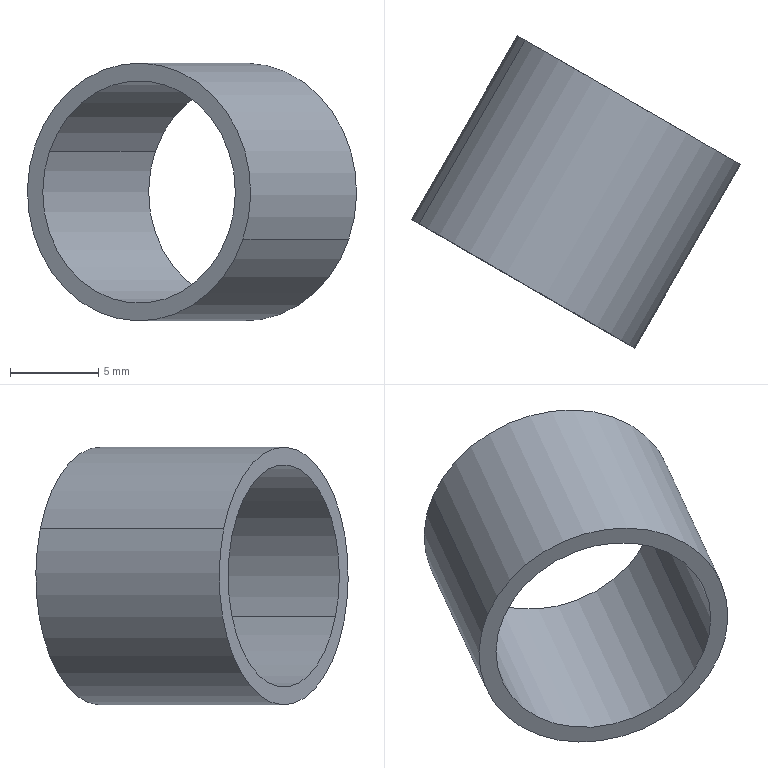Part | SolidWorks | features BaseBody 1 | 1 solid | 6 faces | box 18.644 x 17.692 x 14.6 mm | volume 512.708 mm3 | cylinder 4 | plane 2 | commonest cylinder face diameters 12.6 x2 14.6 x2
STEP:
#1=CARTESIAN_POINT('',(325.471,269.362,2.3));
#2=VERTEX_POINT('',#1);
#3=CARTESIAN_POINT('',(335.629,263.497,-2.3));
#4=VERTEX_POINT('',#3);
#5=CARTESIAN_POINT('',(330.55,266.429,0.));
#6=DIRECTION('',(-0.5,-0.866,0.));
#7=DIRECTION('',(0.8063,-0.4655,-0.365));
#8=AXIS2_PLACEMENT_3D('',#5,#6,#7);
#9=CIRCLE('',#8,6.3);
#10=EDGE_CURVE('',#2,#4,#9,.T.);
#11=ORIENTED_EDGE('',*,*,#10,.T.);
#12=CARTESIAN_POINT('',(341.629,273.889,-2.3));
#13=VERTEX_POINT('',#12);
#14=CARTESIAN_POINT('',(335.629,263.497,-2.3));
#15=DIRECTION('',(0.5,0.866,0.));
#16=VECTOR('',#15,1000.);
#17=LINE('',#14,#16);
#18=EDGE_CURVE('',#4,#13,#17,.T.);
#19=ORIENTED_EDGE('',*,*,#18,.T.);
#20=CARTESIAN_POINT('',(331.471,279.754,2.3));
#21=VERTEX_POINT('',#20);
#22=CARTESIAN_POINT('',(336.55,276.821,0.));
#23=DIRECTION('',(-0.5,-0.866,0.));
#24=DIRECTION('',(0.8063,-0.4655,-0.365));
#25=AXIS2_PLACEMENT_3D('',#22,#23,#24);
#26=CIRCLE('',#25,6.3);
#27=EDGE_CURVE('',#21,#13,#26,.T.);
#28=ORIENTED_EDGE('',*,*,#27,.F.);
#29=CARTESIAN_POINT('',(325.471,269.362,2.3));
#30=DIRECTION('',(0.5,0.866,0.));
#31=VECTOR('',#30,1000.);
#32=LINE('',#29,#31);
#33=EDGE_CURVE('',#2,#21,#32,.T.);
#34=ORIENTED_EDGE('',*,*,#33,.F.);
#35=EDGE_LOOP('',(#11,#19,#28,#34));
#36=FACE_OUTER_BOUND('',#35,.T.);
#37=CARTESIAN_POINT('',(330.55,266.429,0.));
#38=DIRECTION('',(0.5,0.866,0.));
#39=DIRECTION('',(-0.8063,0.4655,0.365));
#40=AXIS2_PLACEMENT_3D('',#37,#38,#39);
#41=CYLINDRICAL_SURFACE('',#40,6.3);
#42=ADVANCED_FACE('',(#36),#41,.F.);
#43=CARTESIAN_POINT('',(336.436,263.031,-2.665));
#44=VERTEX_POINT('',#43);
#45=CARTESIAN_POINT('',(324.664,269.827,2.665));
#46=VERTEX_POINT('',#45);
#47=CARTESIAN_POINT('',(330.55,266.429,0.));
#48=DIRECTION('',(-0.5,-0.866,0.));
#49=DIRECTION('',(0.8063,-0.4655,-0.365));
#50=AXIS2_PLACEMENT_3D('',#47,#48,#49);
#51=CIRCLE('',#50,7.3);
#52=EDGE_CURVE('',#44,#46,#51,.T.);
#53=ORIENTED_EDGE('',*,*,#52,.F.);
#54=CARTESIAN_POINT('',(342.436,273.423,-2.665));
#55=VERTEX_POINT('',#54);
#56=CARTESIAN_POINT('',(336.436,263.031,-2.665));
#57=DIRECTION('',(0.5,0.866,0.));
#58=VECTOR('',#57,1000.);
#59=LINE('',#56,#58);
#60=EDGE_CURVE('',#44,#55,#59,.T.);
#61=ORIENTED_EDGE('',*,*,#60,.T.);
#62=CARTESIAN_POINT('',(330.664,280.22,2.665));
#63=VERTEX_POINT('',#62);
#64=CARTESIAN_POINT('',(336.55,276.821,0.));
#65=DIRECTION('',(-0.5,-0.866,0.));
#66=DIRECTION('',(0.8063,-0.4655,-0.365));
#67=AXIS2_PLACEMENT_3D('',#64,#65,#66);
#68=CIRCLE('',#67,7.3);
#69=EDGE_CURVE('',#55,#63,#68,.T.);
#70=ORIENTED_EDGE('',*,*,#69,.T.);
#71=CARTESIAN_POINT('',(324.664,269.827,2.665));
#72=DIRECTION('',(0.5,0.866,0.));
#73=VECTOR('',#72,1000.);
#74=LINE('',#71,#73);
#75=EDGE_CURVE('',#46,#63,#74,.T.);
#76=ORIENTED_EDGE('',*,*,#75,.F.);
#77=EDGE_LOOP('',(#53,#61,#70,#76));
#78=FACE_OUTER_BOUND('',#77,.T.);
#79=CARTESIAN_POINT('',(330.55,266.429,0.));
#80=DIRECTION('',(0.5,0.866,0.));
#81=DIRECTION('',(-0.8063,0.4655,0.365));
#82=AXIS2_PLACEMENT_3D('',#79,#80,#81);
#83=CYLINDRICAL_SURFACE('',#82,7.3);
#84=ADVANCED_FACE('',(#78),#83,.T.);
#85=CARTESIAN_POINT('',(330.55,266.429,0.));
#86=DIRECTION('',(-0.5,-0.866,0.));
#87=DIRECTION('',(0.8063,-0.4655,-0.365));
#88=AXIS2_PLACEMENT_3D('',#85,#86,#87);
#89=CIRCLE('',#88,7.3);
#90=EDGE_CURVE('',#46,#44,#89,.T.);
#91=ORIENTED_EDGE('',*,*,#90,.T.);
#92=ORIENTED_EDGE('',*,*,#52,.T.);
#93=EDGE_LOOP('',(#91,#92));
#94=FACE_OUTER_BOUND('',#93,.T.);
#95=ORIENTED_EDGE('',*,*,#10,.F.);
#96=CARTESIAN_POINT('',(330.55,266.429,0.));
#97=DIRECTION('',(-0.5,-0.866,0.));
#98=DIRECTION('',(0.8063,-0.4655,-0.365));
#99=AXIS2_PLACEMENT_3D('',#96,#97,#98);
#100=CIRCLE('',#99,6.3);
#101=EDGE_CURVE('',#4,#2,#100,.T.);
#102=ORIENTED_EDGE('',*,*,#101,.F.);
#103=EDGE_LOOP('',(#95,#102));
#104=FACE_BOUND('',#103,.T.);
#105=CARTESIAN_POINT('',(330.55,266.429,0.));
#106=DIRECTION('',(-0.5,-0.866,0.));
#107=DIRECTION('',(0.8063,-0.4655,-0.365));
#108=AXIS2_PLACEMENT_3D('',#105,#106,#107);
#109=PLANE('',#108);
#110=ADVANCED_FACE('',(#94,#104),#109,.T.);
#111=CARTESIAN_POINT('',(336.55,276.821,0.));
#112=DIRECTION('',(-0.5,-0.866,0.));
#113=DIRECTION('',(0.8063,-0.4655,-0.365));
#114=AXIS2_PLACEMENT_3D('',#111,#112,#113);
#115=CIRCLE('',#114,7.3);
#116=EDGE_CURVE('',#63,#55,#115,.T.);
#117=ORIENTED_EDGE('',*,*,#116,.F.);
#118=ORIENTED_EDGE('',*,*,#69,.F.);
#119=EDGE_LOOP('',(#117,#118));
#120=FACE_OUTER_BOUND('',#119,.T.);
#121=ORIENTED_EDGE('',*,*,#27,.T.);
#122=CARTESIAN_POINT('',(336.55,276.821,0.));
#123=DIRECTION('',(-0.5,-0.866,0.));
#124=DIRECTION('',(0.8063,-0.4655,-0.365));
#125=AXIS2_PLACEMENT_3D('',#122,#123,#124);
#126=CIRCLE('',#125,6.3);
#127=EDGE_CURVE('',#13,#21,#126,.T.);
#128=ORIENTED_EDGE('',*,*,#127,.T.);
#129=EDGE_LOOP('',(#121,#128));
#130=FACE_BOUND('',#129,.T.);
#131=CARTESIAN_POINT('',(336.55,276.821,0.));
#132=DIRECTION('',(-0.5,-0.866,0.));
#133=DIRECTION('',(0.8063,-0.4655,-0.365));
#134=AXIS2_PLACEMENT_3D('',#131,#132,#133);
#135=PLANE('',#134);
#136=ADVANCED_FACE('',(#120,#130),#135,.F.);
#137=ORIENTED_EDGE('',*,*,#60,.F.);
#138=ORIENTED_EDGE('',*,*,#90,.F.);
#139=ORIENTED_EDGE('',*,*,#75,.T.);
#140=ORIENTED_EDGE('',*,*,#116,.T.);
#141=EDGE_LOOP('',(#137,#138,#139,#140));
#142=FACE_OUTER_BOUND('',#141,.T.);
#143=CARTESIAN_POINT('',(330.55,266.429,0.));
#144=DIRECTION('',(0.5,0.866,0.));
#145=DIRECTION('',(-0.8063,0.4655,0.365));
#146=AXIS2_PLACEMENT_3D('',#143,#144,#145);
#147=CYLINDRICAL_SURFACE('',#146,7.3);
#148=ADVANCED_FACE('',(#142),#147,.T.);
#149=ORIENTED_EDGE('',*,*,#18,.F.);
#150=ORIENTED_EDGE('',*,*,#101,.T.);
#151=ORIENTED_EDGE('',*,*,#33,.T.);
#152=ORIENTED_EDGE('',*,*,#127,.F.);
#153=EDGE_LOOP('',(#149,#150,#151,#152));
#154=FACE_OUTER_BOUND('',#153,.T.);
#155=CARTESIAN_POINT('',(330.55,266.429,0.));
#156=DIRECTION('',(0.5,0.866,0.));
#157=DIRECTION('',(-0.8063,0.4655,0.365));
#158=AXIS2_PLACEMENT_3D('',#155,#156,#157);
#159=CYLINDRICAL_SURFACE('',#158,6.3);
#160=ADVANCED_FACE('',(#154),#159,.F.);
#161=CLOSED_SHELL('',(#42,#84,#110,#136,#148,#160));
#162=MANIFOLD_SOLID_BREP('',#161);
#163=CARTESIAN_POINT('',(0.,0.,0.));
#164=DIRECTION('',(0.,0.,1.));
#165=DIRECTION('',(1.,0.,0.));
#166=AXIS2_PLACEMENT_3D('',#163,#164,#165);
#167=(LENGTH_UNIT()NAMED_UNIT(*)SI_UNIT(.MILLI.,.METRE.));
#168=UNCERTAINTY_MEASURE_WITH_UNIT(LENGTH_MEASURE(0.00001),#167,'','');
#169=(NAMED_UNIT(*)PLANE_ANGLE_UNIT()SI_UNIT($,.RADIAN.));
#170=(NAMED_UNIT(*)SI_UNIT($,.STERADIAN.)SOLID_ANGLE_UNIT());
#171=(GEOMETRIC_REPRESENTATION_CONTEXT(3)GLOBAL_UNCERTAINTY_ASSIGNED_CONTEXT((#168))GLOBAL_UNIT_ASSIGNED_CONTEXT((#167,#169,#170))REPRESENTATION_CONTEXT('',''));
#172=ADVANCED_BREP_SHAPE_REPRESENTATION('',(#162,#166),#171);